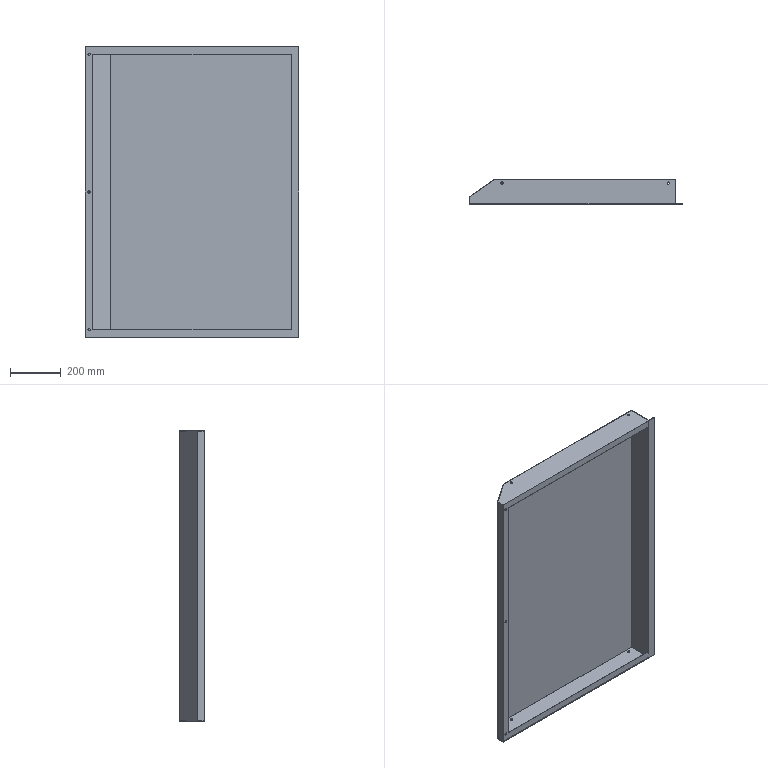Part | SolidWorks | features ICE 5, Extrusion 1, Shell 1 | 1 solid | 37 faces | box 841 x 100 x 1142 mm | volume 2713356 mm3 | plane 19 | cylinder 18 | commonest cylinder face diameters 9 x18
STEP:
#1=CARTESIAN_POINT('',(-2.,84.,482.5));
#2=VERTEX_POINT('',#1);
#3=CARTESIAN_POINT('',(-2.,84.,491.5));
#4=VERTEX_POINT('',#3);
#5=CARTESIAN_POINT('',(-2.,84.,487.));
#6=DIRECTION('',(-1.,0.,0.));
#7=DIRECTION('',(0.,0.,1.));
#8=AXIS2_PLACEMENT_3D('',#5,#6,#7);
#9=CIRCLE('',#8,4.5);
#10=EDGE_CURVE('',#2,#4,#9,.T.);
#11=ORIENTED_EDGE('',*,*,#10,.T.);
#12=CARTESIAN_POINT('',(0.,84.,491.5));
#13=VERTEX_POINT('',#12);
#14=CARTESIAN_POINT('',(-10.,84.,491.5));
#15=DIRECTION('',(1.,0.,0.));
#16=VECTOR('',#15,1000.);
#17=LINE('',#14,#16);
#18=EDGE_CURVE('',#4,#13,#17,.T.);
#19=ORIENTED_EDGE('',*,*,#18,.T.);
#20=CARTESIAN_POINT('',(0.,84.,482.5));
#21=VERTEX_POINT('',#20);
#22=CARTESIAN_POINT('',(0.,84.,487.));
#23=DIRECTION('',(1.,0.,0.));
#24=DIRECTION('',(0.,0.,-1.));
#25=AXIS2_PLACEMENT_3D('',#22,#23,#24);
#26=CIRCLE('',#25,4.5);
#27=EDGE_CURVE('',#13,#21,#26,.T.);
#28=ORIENTED_EDGE('',*,*,#27,.T.);
#29=CARTESIAN_POINT('',(-10.,84.,482.5));
#30=DIRECTION('',(1.,0.,0.));
#31=VECTOR('',#30,1000.);
#32=LINE('',#29,#31);
#33=EDGE_CURVE('',#2,#21,#32,.T.);
#34=ORIENTED_EDGE('',*,*,#33,.F.);
#35=EDGE_LOOP('',(#11,#19,#28,#34));
#36=FACE_OUTER_BOUND('',#35,.T.);
#37=CARTESIAN_POINT('',(-10.,84.,487.));
#38=DIRECTION('',(1.,0.,0.));
#39=DIRECTION('',(0.,0.,-1.));
#40=AXIS2_PLACEMENT_3D('',#37,#38,#39);
#41=CYLINDRICAL_SURFACE('',#40,4.5);
#42=ADVANCED_FACE('',(#36),#41,.F.);
#43=CARTESIAN_POINT('',(-2.,84.,550.5));
#44=VERTEX_POINT('',#43);
#45=CARTESIAN_POINT('',(-2.,84.,559.5));
#46=VERTEX_POINT('',#45);
#47=CARTESIAN_POINT('',(-2.,84.,555.));
#48=DIRECTION('',(-1.,0.,0.));
#49=DIRECTION('',(0.,0.,1.));
#50=AXIS2_PLACEMENT_3D('',#47,#48,#49);
#51=CIRCLE('',#50,4.5);
#52=EDGE_CURVE('',#44,#46,#51,.T.);
#53=ORIENTED_EDGE('',*,*,#52,.T.);
#54=CARTESIAN_POINT('',(0.,84.,559.5));
#55=VERTEX_POINT('',#54);
#56=CARTESIAN_POINT('',(-10.,84.,559.5));
#57=DIRECTION('',(1.,0.,0.));
#58=VECTOR('',#57,1000.);
#59=LINE('',#56,#58);
#60=EDGE_CURVE('',#46,#55,#59,.T.);
#61=ORIENTED_EDGE('',*,*,#60,.T.);
#62=CARTESIAN_POINT('',(0.,84.,550.5));
#63=VERTEX_POINT('',#62);
#64=CARTESIAN_POINT('',(0.,84.,555.));
#65=DIRECTION('',(1.,0.,0.));
#66=DIRECTION('',(0.,0.,-1.));
#67=AXIS2_PLACEMENT_3D('',#64,#65,#66);
#68=CIRCLE('',#67,4.5);
#69=EDGE_CURVE('',#55,#63,#68,.T.);
#70=ORIENTED_EDGE('',*,*,#69,.T.);
#71=CARTESIAN_POINT('',(-10.,84.,550.5));
#72=DIRECTION('',(1.,0.,0.));
#73=VECTOR('',#72,1000.);
#74=LINE('',#71,#73);
#75=EDGE_CURVE('',#44,#63,#74,.T.);
#76=ORIENTED_EDGE('',*,*,#75,.F.);
#77=EDGE_LOOP('',(#53,#61,#70,#76));
#78=FACE_OUTER_BOUND('',#77,.T.);
#79=CARTESIAN_POINT('',(-10.,84.,555.));
#80=DIRECTION('',(1.,0.,0.));
#81=DIRECTION('',(0.,0.,-1.));
#82=AXIS2_PLACEMENT_3D('',#79,#80,#81);
#83=CYLINDRICAL_SURFACE('',#82,4.5);
#84=ADVANCED_FACE('',(#78),#83,.F.);
#85=CARTESIAN_POINT('',(-801.5,2.,0.));
#86=VERTEX_POINT('',#85);
#87=CARTESIAN_POINT('',(-792.5,2.,0.));
#88=VERTEX_POINT('',#87);
#89=CARTESIAN_POINT('',(-797.,2.,0.));
#90=DIRECTION('',(0.,-1.,0.));
#91=DIRECTION('',(1.,0.,0.));
#92=AXIS2_PLACEMENT_3D('',#89,#90,#91);
#93=CIRCLE('',#92,4.5);
#94=EDGE_CURVE('',#86,#88,#93,.T.);
#95=ORIENTED_EDGE('',*,*,#94,.F.);
#96=CARTESIAN_POINT('',(-801.5,0.,0.));
#97=VERTEX_POINT('',#96);
#98=CARTESIAN_POINT('',(-801.5,2.,0.));
#99=DIRECTION('',(0.,-1.,0.));
#100=VECTOR('',#99,1000.);
#101=LINE('',#98,#100);
#102=EDGE_CURVE('',#86,#97,#101,.T.);
#103=ORIENTED_EDGE('',*,*,#102,.T.);
#104=CARTESIAN_POINT('',(-792.5,0.,0.));
#105=VERTEX_POINT('',#104);
#106=CARTESIAN_POINT('',(-797.,0.,0.));
#107=DIRECTION('',(0.,-1.,0.));
#108=DIRECTION('',(1.,0.,0.));
#109=AXIS2_PLACEMENT_3D('',#106,#107,#108);
#110=CIRCLE('',#109,4.5);
#111=EDGE_CURVE('',#97,#105,#110,.T.);
#112=ORIENTED_EDGE('',*,*,#111,.T.);
#113=CARTESIAN_POINT('',(-792.5,2.,0.));
#114=DIRECTION('',(0.,-1.,0.));
#115=VECTOR('',#114,1000.);
#116=LINE('',#113,#115);
#117=EDGE_CURVE('',#88,#105,#116,.T.);
#118=ORIENTED_EDGE('',*,*,#117,.F.);
#119=EDGE_LOOP('',(#95,#103,#112,#118));
#120=FACE_OUTER_BOUND('',#119,.T.);
#121=CARTESIAN_POINT('',(-797.,2.,0.));
#122=DIRECTION('',(0.,-1.,0.));
#123=DIRECTION('',(1.,0.,0.));
#124=AXIS2_PLACEMENT_3D('',#121,#122,#123);
#125=CYLINDRICAL_SURFACE('',#124,4.5);
#126=ADVANCED_FACE('',(#120),#125,.F.);
#127=CARTESIAN_POINT('',(-801.5,2.,-541.));
#128=VERTEX_POINT('',#127);
#129=CARTESIAN_POINT('',(-792.5,2.,-541.));
#130=VERTEX_POINT('',#129);
#131=CARTESIAN_POINT('',(-797.,2.,-541.));
#132=DIRECTION('',(0.,-1.,0.));
#133=DIRECTION('',(1.,0.,0.));
#134=AXIS2_PLACEMENT_3D('',#131,#132,#133);
#135=CIRCLE('',#134,4.5);
#136=EDGE_CURVE('',#128,#130,#135,.T.);
#137=ORIENTED_EDGE('',*,*,#136,.F.);
#138=CARTESIAN_POINT('',(-801.5,0.,-541.));
#139=VERTEX_POINT('',#138);
#140=CARTESIAN_POINT('',(-801.5,2.,-541.));
#141=DIRECTION('',(0.,-1.,0.));
#142=VECTOR('',#141,1000.);
#143=LINE('',#140,#142);
#144=EDGE_CURVE('',#128,#139,#143,.T.);
#145=ORIENTED_EDGE('',*,*,#144,.T.);
#146=CARTESIAN_POINT('',(-792.5,0.,-541.));
#147=VERTEX_POINT('',#146);
#148=CARTESIAN_POINT('',(-797.,0.,-541.));
#149=DIRECTION('',(0.,-1.,0.));
#150=DIRECTION('',(1.,0.,0.));
#151=AXIS2_PLACEMENT_3D('',#148,#149,#150);
#152=CIRCLE('',#151,4.5);
#153=EDGE_CURVE('',#139,#147,#152,.T.);
#154=ORIENTED_EDGE('',*,*,#153,.T.);
#155=CARTESIAN_POINT('',(-792.5,2.,-541.));
#156=DIRECTION('',(0.,-1.,0.));
#157=VECTOR('',#156,1000.);
#158=LINE('',#155,#157);
#159=EDGE_CURVE('',#130,#147,#158,.T.);
#160=ORIENTED_EDGE('',*,*,#159,.F.);
#161=EDGE_LOOP('',(#137,#145,#154,#160));
#162=FACE_OUTER_BOUND('',#161,.T.);
#163=CARTESIAN_POINT('',(-797.,2.,-541.));
#164=DIRECTION('',(0.,-1.,0.));
#165=DIRECTION('',(1.,0.,0.));
#166=AXIS2_PLACEMENT_3D('',#163,#164,#165);
#167=CYLINDRICAL_SURFACE('',#166,4.5);
#168=ADVANCED_FACE('',(#162),#167,.F.);
#169=CARTESIAN_POINT('',(-801.5,2.,541.));
#170=VERTEX_POINT('',#169);
#171=CARTESIAN_POINT('',(-792.5,2.,541.));
#172=VERTEX_POINT('',#171);
#173=CARTESIAN_POINT('',(-797.,2.,541.));
#174=DIRECTION('',(0.,-1.,0.));
#175=DIRECTION('',(1.,0.,0.));
#176=AXIS2_PLACEMENT_3D('',#173,#174,#175);
#177=CIRCLE('',#176,4.5);
#178=EDGE_CURVE('',#170,#172,#177,.T.);
#179=ORIENTED_EDGE('',*,*,#178,.F.);
#180=CARTESIAN_POINT('',(-801.5,0.,541.));
#181=VERTEX_POINT('',#180);
#182=CARTESIAN_POINT('',(-801.5,2.,541.));
#183=DIRECTION('',(0.,-1.,0.));
#184=VECTOR('',#183,1000.);
#185=LINE('',#182,#184);
#186=EDGE_CURVE('',#170,#181,#185,.T.);
#187=ORIENTED_EDGE('',*,*,#186,.T.);
#188=CARTESIAN_POINT('',(-792.5,0.,541.));
#189=VERTEX_POINT('',#188);
#190=CARTESIAN_POINT('',(-797.,0.,541.));
#191=DIRECTION('',(0.,-1.,0.));
#192=DIRECTION('',(1.,0.,0.));
#193=AXIS2_PLACEMENT_3D('',#190,#191,#192);
#194=CIRCLE('',#193,4.5);
#195=EDGE_CURVE('',#181,#189,#194,.T.);
#196=ORIENTED_EDGE('',*,*,#195,.T.);
#197=CARTESIAN_POINT('',(-792.5,2.,541.));
#198=DIRECTION('',(0.,-1.,0.));
#199=VECTOR('',#198,1000.);
#200=LINE('',#197,#199);
#201=EDGE_CURVE('',#172,#189,#200,.T.);
#202=ORIENTED_EDGE('',*,*,#201,.F.);
#203=EDGE_LOOP('',(#179,#187,#196,#202));
#204=FACE_OUTER_BOUND('',#203,.T.);
#205=CARTESIAN_POINT('',(-797.,2.,541.));
#206=DIRECTION('',(0.,-1.,0.));
#207=DIRECTION('',(1.,0.,0.));
#208=AXIS2_PLACEMENT_3D('',#205,#206,#207);
#209=CYLINDRICAL_SURFACE('',#208,4.5);
#210=ADVANCED_FACE('',(#204),#209,.F.);
#211=CARTESIAN_POINT('',(-34.5,84.,569.));
#212=VERTEX_POINT('',#211);
#213=CARTESIAN_POINT('',(-25.5,84.,569.));
#214=VERTEX_POINT('',#213);
#215=CARTESIAN_POINT('',(-30.,84.,569.));
#216=DIRECTION('',(0.,0.,1.));
#217=DIRECTION('',(1.,0.,0.));
#218=AXIS2_PLACEMENT_3D('',#215,#216,#217);
#219=CIRCLE('',#218,4.5);
#220=EDGE_CURVE('',#212,#214,#219,.T.);
#221=ORIENTED_EDGE('',*,*,#220,.F.);
#222=CARTESIAN_POINT('',(-34.5,84.,571.));
#223=VERTEX_POINT('',#222);
#224=CARTESIAN_POINT('',(-34.5,84.,-604.));
#225=DIRECTION('',(0.,0.,1.));
#226=VECTOR('',#225,1000.);
#227=LINE('',#224,#226);
#228=EDGE_CURVE('',#212,#223,#227,.T.);
#229=ORIENTED_EDGE('',*,*,#228,.T.);
#230=CARTESIAN_POINT('',(-25.5,84.,571.));
#231=VERTEX_POINT('',#230);
#232=CARTESIAN_POINT('',(-30.,84.,571.));
#233=DIRECTION('',(0.,0.,1.));
#234=DIRECTION('',(1.,0.,0.));
#235=AXIS2_PLACEMENT_3D('',#232,#233,#234);
#236=CIRCLE('',#235,4.5);
#237=EDGE_CURVE('',#223,#231,#236,.T.);
#238=ORIENTED_EDGE('',*,*,#237,.T.);
#239=CARTESIAN_POINT('',(-25.5,84.,-604.));
#240=DIRECTION('',(0.,0.,1.));
#241=VECTOR('',#240,1000.);
#242=LINE('',#239,#241);
#243=EDGE_CURVE('',#214,#231,#242,.T.);
#244=ORIENTED_EDGE('',*,*,#243,.F.);
#245=EDGE_LOOP('',(#221,#229,#238,#244));
#246=FACE_OUTER_BOUND('',#245,.T.);
#247=CARTESIAN_POINT('',(-30.,84.,-604.));
#248=DIRECTION('',(0.,0.,1.));
#249=DIRECTION('',(1.,0.,0.));
#250=AXIS2_PLACEMENT_3D('',#247,#248,#249);
#251=CYLINDRICAL_SURFACE('',#250,4.5);
#252=ADVANCED_FACE('',(#246),#251,.F.);
#253=CARTESIAN_POINT('',(-34.5,84.,-571.));
#254=VERTEX_POINT('',#253);
#255=CARTESIAN_POINT('',(-25.5,84.,-571.));
#256=VERTEX_POINT('',#255);
#257=CARTESIAN_POINT('',(-30.,84.,-571.));
#258=DIRECTION('',(0.,0.,1.));
#259=DIRECTION('',(1.,0.,0.));
#260=AXIS2_PLACEMENT_3D('',#257,#258,#259);
#261=CIRCLE('',#260,4.5);
#262=EDGE_CURVE('',#254,#256,#261,.T.);
#263=ORIENTED_EDGE('',*,*,#262,.F.);
#264=CARTESIAN_POINT('',(-34.5,84.,-569.));
#265=VERTEX_POINT('',#264);
#266=CARTESIAN_POINT('',(-34.5,84.,-604.));
#267=DIRECTION('',(0.,0.,1.));
#268=VECTOR('',#267,1000.);
#269=LINE('',#266,#268);
#270=EDGE_CURVE('',#254,#265,#269,.T.);
#271=ORIENTED_EDGE('',*,*,#270,.T.);
#272=CARTESIAN_POINT('',(-25.5,84.,-569.));
#273=VERTEX_POINT('',#272);
#274=CARTESIAN_POINT('',(-30.,84.,-569.));
#275=DIRECTION('',(0.,0.,1.));
#276=DIRECTION('',(1.,0.,0.));
#277=AXIS2_PLACEMENT_3D('',#274,#275,#276);
#278=CIRCLE('',#277,4.5);
#279=EDGE_CURVE('',#265,#273,#278,.T.);
#280=ORIENTED_EDGE('',*,*,#279,.T.);
#281=CARTESIAN_POINT('',(-25.5,84.,-604.));
#282=DIRECTION('',(0.,0.,1.));
#283=VECTOR('',#282,1000.);
#284=LINE('',#281,#283);
#285=EDGE_CURVE('',#256,#273,#284,.T.);
#286=ORIENTED_EDGE('',*,*,#285,.F.);
#287=EDGE_LOOP('',(#263,#271,#280,#286));
#288=FACE_OUTER_BOUND('',#287,.T.);
#289=CARTESIAN_POINT('',(-30.,84.,-604.));
#290=DIRECTION('',(0.,0.,1.));
#291=DIRECTION('',(1.,0.,0.));
#292=AXIS2_PLACEMENT_3D('',#289,#290,#291);
#293=CYLINDRICAL_SURFACE('',#292,4.5);
#294=ADVANCED_FACE('',(#288),#293,.F.);
#295=CARTESIAN_POINT('',(-687.53,84.,569.));
#296=VERTEX_POINT('',#295);
#297=CARTESIAN_POINT('',(-678.53,84.,569.));
#298=VERTEX_POINT('',#297);
#299=CARTESIAN_POINT('',(-683.03,84.,569.));
#300=DIRECTION('',(0.,0.,1.));
#301=DIRECTION('',(1.,0.,0.));
#302=AXIS2_PLACEMENT_3D('',#299,#300,#301);
#303=CIRCLE('',#302,4.5);
#304=EDGE_CURVE('',#296,#298,#303,.T.);
#305=ORIENTED_EDGE('',*,*,#304,.F.);
#306=CARTESIAN_POINT('',(-687.53,84.,571.));
#307=VERTEX_POINT('',#306);
#308=CARTESIAN_POINT('',(-687.53,84.,-604.));
#309=DIRECTION('',(0.,0.,1.));
#310=VECTOR('',#309,1000.);
#311=LINE('',#308,#310);
#312=EDGE_CURVE('',#296,#307,#311,.T.);
#313=ORIENTED_EDGE('',*,*,#312,.T.);
#314=CARTESIAN_POINT('',(-678.53,84.,571.));
#315=VERTEX_POINT('',#314);
#316=CARTESIAN_POINT('',(-683.03,84.,571.));
#317=DIRECTION('',(0.,0.,1.));
#318=DIRECTION('',(1.,0.,0.));
#319=AXIS2_PLACEMENT_3D('',#316,#317,#318);
#320=CIRCLE('',#319,4.5);
#321=EDGE_CURVE('',#307,#315,#320,.T.);
#322=ORIENTED_EDGE('',*,*,#321,.T.);
#323=CARTESIAN_POINT('',(-678.53,84.,-604.));
#324=DIRECTION('',(0.,0.,1.));
#325=VECTOR('',#324,1000.);
#326=LINE('',#323,#325);
#327=EDGE_CURVE('',#298,#315,#326,.T.);
#328=ORIENTED_EDGE('',*,*,#327,.F.);
#329=EDGE_LOOP('',(#305,#313,#322,#328));
#330=FACE_OUTER_BOUND('',#329,.T.);
#331=CARTESIAN_POINT('',(-683.03,84.,-604.));
#332=DIRECTION('',(0.,0.,1.));
#333=DIRECTION('',(1.,0.,0.));
#334=AXIS2_PLACEMENT_3D('',#331,#332,#333);
#335=CYLINDRICAL_SURFACE('',#334,4.5);
#336=ADVANCED_FACE('',(#330),#335,.F.);
#337=CARTESIAN_POINT('',(-687.53,84.,-571.));
#338=VERTEX_POINT('',#337);
#339=CARTESIAN_POINT('',(-678.53,84.,-571.));
#340=VERTEX_POINT('',#339);
#341=CARTESIAN_POINT('',(-683.03,84.,-571.));
#342=DIRECTION('',(0.,0.,1.));
#343=DIRECTION('',(1.,0.,0.));
#344=AXIS2_PLACEMENT_3D('',#341,#342,#343);
#345=CIRCLE('',#344,4.5);
#346=EDGE_CURVE('',#338,#340,#345,.T.);
#347=ORIENTED_EDGE('',*,*,#346,.F.);
#348=CARTESIAN_POINT('',(-687.53,84.,-569.));
#349=VERTEX_POINT('',#348);
#350=CARTESIAN_POINT('',(-687.53,84.,-604.));
#351=DIRECTION('',(0.,0.,1.));
#352=VECTOR('',#351,1000.);
#353=LINE('',#350,#352);
#354=EDGE_CURVE('',#338,#349,#353,.T.);
#355=ORIENTED_EDGE('',*,*,#354,.T.);
#356=CARTESIAN_POINT('',(-678.53,84.,-569.));
#357=VERTEX_POINT('',#356);
#358=CARTESIAN_POINT('',(-683.03,84.,-569.));
#359=DIRECTION('',(0.,0.,1.));
#360=DIRECTION('',(1.,0.,0.));
#361=AXIS2_PLACEMENT_3D('',#358,#359,#360);
#362=CIRCLE('',#361,4.5);
#363=EDGE_CURVE('',#349,#357,#362,.T.);
#364=ORIENTED_EDGE('',*,*,#363,.T.);
#365=CARTESIAN_POINT('',(-678.53,84.,-604.));
#366=DIRECTION('',(0.,0.,1.));
#367=VECTOR('',#366,1000.);
#368=LINE('',#365,#367);
#369=EDGE_CURVE('',#340,#357,#368,.T.);
#370=ORIENTED_EDGE('',*,*,#369,.F.);
#371=EDGE_LOOP('',(#347,#355,#364,#370));
#372=FACE_OUTER_BOUND('',#371,.T.);
#373=CARTESIAN_POINT('',(-683.03,84.,-604.));
#374=DIRECTION('',(0.,0.,1.));
#375=DIRECTION('',(1.,0.,0.));
#376=AXIS2_PLACEMENT_3D('',#373,#374,#375);
#377=CYLINDRICAL_SURFACE('',#376,4.5);
#378=ADVANCED_FACE('',(#372),#377,.F.);
#379=CARTESIAN_POINT('',(-811.,28.959,569.));
#380=VERTEX_POINT('',#379);
#381=CARTESIAN_POINT('',(-811.,2.,569.));
#382=VERTEX_POINT('',#381);
#383=CARTESIAN_POINT('',(-811.,0.,569.));
#384=DIRECTION('',(0.,-1.,0.));
#385=VECTOR('',#384,1000.);
#386=LINE('',#383,#385);
#387=EDGE_CURVE('',#380,#382,#386,.T.);
#388=ORIENTED_EDGE('',*,*,#387,.T.);
#389=CARTESIAN_POINT('',(-811.,2.,-569.));
#390=VERTEX_POINT('',#389);
#391=CARTESIAN_POINT('',(-811.,2.,571.));
#392=DIRECTION('',(0.,0.,-1.));
#393=VECTOR('',#392,1000.);
#394=LINE('',#391,#393);
#395=EDGE_CURVE('',#382,#390,#394,.T.);
#396=ORIENTED_EDGE('',*,*,#395,.T.);
#397=CARTESIAN_POINT('',(-811.,28.959,-569.));
#398=VERTEX_POINT('',#397);
#399=CARTESIAN_POINT('',(-811.,0.,-569.));
#400=DIRECTION('',(0.,-1.,0.));
#401=VECTOR('',#400,1000.);
#402=LINE('',#399,#401);
#403=EDGE_CURVE('',#398,#390,#402,.T.);
#404=ORIENTED_EDGE('',*,*,#403,.F.);
#405=CARTESIAN_POINT('',(-811.,28.959,571.));
#406=DIRECTION('',(0.,0.,-1.));
#407=VECTOR('',#406,1000.);
#408=LINE('',#405,#407);
#409=EDGE_CURVE('',#380,#398,#408,.T.);
#410=ORIENTED_EDGE('',*,*,#409,.F.);
#411=EDGE_LOOP('',(#388,#396,#404,#410));
#412=FACE_OUTER_BOUND('',#411,.T.);
#413=CARTESIAN_POINT('',(-811.,0.,571.));
#414=DIRECTION('',(1.,0.,0.));
#415=DIRECTION('',(0.,1.,0.));
#416=AXIS2_PLACEMENT_3D('',#413,#414,#415);
#417=PLANE('',#416);
#418=ADVANCED_FACE('',(#412),#417,.T.);
#419=CARTESIAN_POINT('',(-683.03,84.,569.));
#420=DIRECTION('',(0.,0.,1.));
#421=DIRECTION('',(1.,0.,0.));
#422=AXIS2_PLACEMENT_3D('',#419,#420,#421);
#423=CIRCLE('',#422,4.5);
#424=EDGE_CURVE('',#298,#296,#423,.T.);
#425=ORIENTED_EDGE('',*,*,#424,.T.);
#426=ORIENTED_EDGE('',*,*,#304,.T.);
#427=EDGE_LOOP('',(#425,#426));
#428=FACE_BOUND('',#427,.T.);
#429=CARTESIAN_POINT('',(-30.,84.,569.));
#430=DIRECTION('',(0.,0.,1.));
#431=DIRECTION('',(1.,0.,0.));
#432=AXIS2_PLACEMENT_3D('',#429,#430,#431);
#433=CIRCLE('',#432,4.5);
#434=EDGE_CURVE('',#214,#212,#433,.T.);
#435=ORIENTED_EDGE('',*,*,#434,.T.);
#436=ORIENTED_EDGE('',*,*,#220,.T.);
#437=EDGE_LOOP('',(#435,#436));
#438=FACE_BOUND('',#437,.T.);
#439=CARTESIAN_POINT('',(-2.,2.,569.));
#440=VERTEX_POINT('',#439);
#441=CARTESIAN_POINT('',(0.,2.,569.));
#442=DIRECTION('',(1.,0.,0.));
#443=VECTOR('',#442,1000.);
#444=LINE('',#441,#443);
#445=EDGE_CURVE('',#382,#440,#444,.T.);
#446=ORIENTED_EDGE('',*,*,#445,.F.);
#447=ORIENTED_EDGE('',*,*,#387,.F.);
#448=CARTESIAN_POINT('',(-712.399,98.,569.));
#449=VERTEX_POINT('',#448);
#450=CARTESIAN_POINT('',(-711.882,98.362,569.));
#451=DIRECTION('',(-0.8192,-0.5736,0.));
#452=VECTOR('',#451,1000.);
#453=LINE('',#450,#452);
#454=EDGE_CURVE('',#449,#380,#453,.T.);
#455=ORIENTED_EDGE('',*,*,#454,.F.);
#456=CARTESIAN_POINT('',(-2.,98.,569.));
#457=VERTEX_POINT('',#456);
#458=CARTESIAN_POINT('',(0.,98.,569.));
#459=DIRECTION('',(-1.,0.,0.));
#460=VECTOR('',#459,1000.);
#461=LINE('',#458,#460);
#462=EDGE_CURVE('',#457,#449,#461,.T.);
#463=ORIENTED_EDGE('',*,*,#462,.F.);
#464=CARTESIAN_POINT('',(-2.,0.,569.));
#465=DIRECTION('',(0.,1.,0.));
#466=VECTOR('',#465,1000.);
#467=LINE('',#464,#466);
#468=EDGE_CURVE('',#440,#457,#467,.T.);
#469=ORIENTED_EDGE('',*,*,#468,.F.);
#470=EDGE_LOOP('',(#446,#447,#455,#463,#469));
#471=FACE_OUTER_BOUND('',#470,.T.);
#472=CARTESIAN_POINT('',(0.,100.,569.));
#473=DIRECTION('',(0.,0.,1.));
#474=DIRECTION('',(1.,0.,0.));
#475=AXIS2_PLACEMENT_3D('',#472,#473,#474);
#476=PLANE('',#475);
#477=ADVANCED_FACE('',(#428,#438,#471),#476,.F.);
#478=CARTESIAN_POINT('',(-683.03,84.,-569.));
#479=DIRECTION('',(0.,0.,1.));
#480=DIRECTION('',(1.,0.,0.));
#481=AXIS2_PLACEMENT_3D('',#478,#479,#480);
#482=CIRCLE('',#481,4.5);
#483=EDGE_CURVE('',#357,#349,#482,.T.);
#484=ORIENTED_EDGE('',*,*,#483,.F.);
#485=ORIENTED_EDGE('',*,*,#363,.F.);
#486=EDGE_LOOP('',(#484,#485));
#487=FACE_BOUND('',#486,.T.);
#488=CARTESIAN_POINT('',(-30.,84.,-569.));
#489=DIRECTION('',(0.,0.,1.));
#490=DIRECTION('',(1.,0.,0.));
#491=AXIS2_PLACEMENT_3D('',#488,#489,#490);
#492=CIRCLE('',#491,4.5);
#493=EDGE_CURVE('',#273,#265,#492,.T.);
#494=ORIENTED_EDGE('',*,*,#493,.F.);
#495=ORIENTED_EDGE('',*,*,#279,.F.);
#496=EDGE_LOOP('',(#494,#495));
#497=FACE_BOUND('',#496,.T.);
#498=ORIENTED_EDGE('',*,*,#403,.T.);
#499=CARTESIAN_POINT('',(-2.,2.,-569.));
#500=VERTEX_POINT('',#499);
#501=CARTESIAN_POINT('',(0.,2.,-569.));
#502=DIRECTION('',(1.,0.,0.));
#503=VECTOR('',#502,1000.);
#504=LINE('',#501,#503);
#505=EDGE_CURVE('',#390,#500,#504,.T.);
#506=ORIENTED_EDGE('',*,*,#505,.T.);
#507=CARTESIAN_POINT('',(-2.,98.,-569.));
#508=VERTEX_POINT('',#507);
#509=CARTESIAN_POINT('',(-2.,0.,-569.));
#510=DIRECTION('',(0.,1.,0.));
#511=VECTOR('',#510,1000.);
#512=LINE('',#509,#511);
#513=EDGE_CURVE('',#500,#508,#512,.T.);
#514=ORIENTED_EDGE('',*,*,#513,.T.);
#515=CARTESIAN_POINT('',(-712.399,98.,-569.));
#516=VERTEX_POINT('',#515);
#517=CARTESIAN_POINT('',(0.,98.,-569.));
#518=DIRECTION('',(-1.,0.,0.));
#519=VECTOR('',#518,1000.);
#520=LINE('',#517,#519);
#521=EDGE_CURVE('',#508,#516,#520,.T.);
#522=ORIENTED_EDGE('',*,*,#521,.T.);
#523=CARTESIAN_POINT('',(-711.882,98.362,-569.));
#524=DIRECTION('',(-0.8192,-0.5736,0.));
#525=VECTOR('',#524,1000.);
#526=LINE('',#523,#525);
#527=EDGE_CURVE('',#516,#398,#526,.T.);
#528=ORIENTED_EDGE('',*,*,#527,.T.);
#529=EDGE_LOOP('',(#498,#506,#514,#522,#528));
#530=FACE_OUTER_BOUND('',#529,.T.);
#531=CARTESIAN_POINT('',(0.,100.,-569.));
#532=DIRECTION('',(0.,0.,1.));
#533=DIRECTION('',(1.,0.,0.));
#534=AXIS2_PLACEMENT_3D('',#531,#532,#533);
#535=PLANE('',#534);
#536=ADVANCED_FACE('',(#487,#497,#530),#535,.T.);
#537=CARTESIAN_POINT('',(0.,84.,487.));
#538=DIRECTION('',(1.,0.,0.));
#539=DIRECTION('',(0.,0.,-1.));
#540=AXIS2_PLACEMENT_3D('',#537,#538,#539);
#541=CIRCLE('',#540,4.5);
#542=EDGE_CURVE('',#21,#13,#541,.T.);
#543=ORIENTED_EDGE('',*,*,#542,.F.);
#544=ORIENTED_EDGE('',*,*,#27,.F.);
#545=EDGE_LOOP('',(#543,#544));
#546=FACE_BOUND('',#545,.T.);
#547=CARTESIAN_POINT('',(0.,84.,555.));
#548=DIRECTION('',(1.,0.,0.));
#549=DIRECTION('',(0.,0.,-1.));
#550=AXIS2_PLACEMENT_3D('',#547,#548,#549);
#551=CIRCLE('',#550,4.5);
#552=EDGE_CURVE('',#63,#55,#551,.T.);
#553=ORIENTED_EDGE('',*,*,#552,.F.);
#554=ORIENTED_EDGE('',*,*,#69,.F.);
#555=EDGE_LOOP('',(#553,#554));
#556=FACE_BOUND('',#555,.T.);
#557=CARTESIAN_POINT('',(0.,2.,-571.));
#558=VERTEX_POINT('',#557);
#559=CARTESIAN_POINT('',(0.,2.,571.));
#560=VERTEX_POINT('',#559);
#561=CARTESIAN_POINT('',(0.,2.,571.));
#562=DIRECTION('',(0.,0.,1.));
#563=VECTOR('',#562,1000.);
#564=LINE('',#561,#563);
#565=EDGE_CURVE('',#558,#560,#564,.T.);
#566=ORIENTED_EDGE('',*,*,#565,.F.);
#567=CARTESIAN_POINT('',(0.,100.,-571.));
#568=VERTEX_POINT('',#567);
#569=CARTESIAN_POINT('',(0.,0.,-571.));
#570=DIRECTION('',(0.,1.,0.));
#571=VECTOR('',#570,1000.);
#572=LINE('',#569,#571);
#573=EDGE_CURVE('',#558,#568,#572,.T.);
#574=ORIENTED_EDGE('',*,*,#573,.T.);
#575=CARTESIAN_POINT('',(0.,100.,571.));
#576=VERTEX_POINT('',#575);
#577=CARTESIAN_POINT('',(0.,100.,571.));
#578=DIRECTION('',(0.,0.,-1.));
#579=VECTOR('',#578,1000.);
#580=LINE('',#577,#579);
#581=EDGE_CURVE('',#576,#568,#580,.T.);
#582=ORIENTED_EDGE('',*,*,#581,.F.);
#583=CARTESIAN_POINT('',(0.,0.,571.));
#584=DIRECTION('',(0.,1.,0.));
#585=VECTOR('',#584,1000.);
#586=LINE('',#583,#585);
#587=EDGE_CURVE('',#560,#576,#586,.T.);
#588=ORIENTED_EDGE('',*,*,#587,.F.);
#589=EDGE_LOOP('',(#566,#574,#582,#588));
#590=FACE_OUTER_BOUND('',#589,.T.);
#591=CARTESIAN_POINT('',(0.,0.,571.));
#592=DIRECTION('',(-1.,0.,0.));
#593=DIRECTION('',(0.,0.,1.));
#594=AXIS2_PLACEMENT_3D('',#591,#592,#593);
#595=PLANE('',#594);
#596=ADVANCED_FACE('',(#546,#556,#590),#595,.F.);
#597=CARTESIAN_POINT('',(-797.,0.,0.));
#598=DIRECTION('',(0.,-1.,0.));
#599=DIRECTION('',(1.,0.,0.));
#600=AXIS2_PLACEMENT_3D('',#597,#598,#599);
#601=CIRCLE('',#600,4.5);
#602=EDGE_CURVE('',#105,#97,#601,.T.);
#603=ORIENTED_EDGE('',*,*,#602,.F.);
#604=ORIENTED_EDGE('',*,*,#111,.F.);
#605=EDGE_LOOP('',(#603,#604));
#606=FACE_BOUND('',#605,.T.);
#607=CARTESIAN_POINT('',(-797.,0.,-541.));
#608=DIRECTION('',(0.,-1.,0.));
#609=DIRECTION('',(1.,0.,0.));
#610=AXIS2_PLACEMENT_3D('',#607,#608,#609);
#611=CIRCLE('',#610,4.5);
#612=EDGE_CURVE('',#147,#139,#611,.T.);
#613=ORIENTED_EDGE('',*,*,#612,.F.);
#614=ORIENTED_EDGE('',*,*,#153,.F.);
#615=EDGE_LOOP('',(#613,#614));
#616=FACE_BOUND('',#615,.T.);
#617=CARTESIAN_POINT('',(-797.,0.,541.));
#618=DIRECTION('',(0.,-1.,0.));
#619=DIRECTION('',(1.,0.,0.));
#620=AXIS2_PLACEMENT_3D('',#617,#618,#619);
#621=CIRCLE('',#620,4.5);
#622=EDGE_CURVE('',#189,#181,#621,.T.);
#623=ORIENTED_EDGE('',*,*,#622,.F.);
#624=ORIENTED_EDGE('',*,*,#195,.F.);
#625=EDGE_LOOP('',(#623,#624));
#626=FACE_BOUND('',#625,.T.);
#627=CARTESIAN_POINT('',(-783.,0.,541.));
#628=VERTEX_POINT('',#627);
#629=CARTESIAN_POINT('',(-2.,0.,541.));
#630=VERTEX_POINT('',#629);
#631=CARTESIAN_POINT('',(-783.,0.,541.));
#632=DIRECTION('',(1.,0.,0.));
#633=VECTOR('',#632,1000.);
#634=LINE('',#631,#633);
#635=EDGE_CURVE('',#628,#630,#634,.T.);
#636=ORIENTED_EDGE('',*,*,#635,.T.);
#637=CARTESIAN_POINT('',(-2.,0.,-541.));
#638=VERTEX_POINT('',#637);
#639=CARTESIAN_POINT('',(-2.,0.,571.));
#640=DIRECTION('',(0.,0.,-1.));
#641=VECTOR('',#640,1000.);
#642=LINE('',#639,#641);
#643=EDGE_CURVE('',#630,#638,#642,.T.);
#644=ORIENTED_EDGE('',*,*,#643,.T.);
#645=CARTESIAN_POINT('',(-783.,0.,-541.));
#646=VERTEX_POINT('',#645);
#647=CARTESIAN_POINT('',(-783.,0.,-541.));
#648=DIRECTION('',(-1.,0.,0.));
#649=VECTOR('',#648,1000.);
#650=LINE('',#647,#649);
#651=EDGE_CURVE('',#638,#646,#650,.T.);
#652=ORIENTED_EDGE('',*,*,#651,.T.);
#653=CARTESIAN_POINT('',(-783.,0.,541.));
#654=DIRECTION('',(0.,0.,1.));
#655=VECTOR('',#654,1000.);
#656=LINE('',#653,#655);
#657=EDGE_CURVE('',#646,#628,#656,.T.);
#658=ORIENTED_EDGE('',*,*,#657,.T.);
#659=EDGE_LOOP('',(#636,#644,#652,#658));
#660=FACE_BOUND('',#659,.T.);
#661=CARTESIAN_POINT('',(28.,0.,-571.));
#662=VERTEX_POINT('',#661);
#663=CARTESIAN_POINT('',(28.,0.,571.));
#664=VERTEX_POINT('',#663);
#665=CARTESIAN_POINT('',(28.,0.,571.));
#666=DIRECTION('',(0.,0.,1.));
#667=VECTOR('',#666,1000.);
#668=LINE('',#665,#667);
#669=EDGE_CURVE('',#662,#664,#668,.T.);
#670=ORIENTED_EDGE('',*,*,#669,.T.);
#671=CARTESIAN_POINT('',(-813.,0.,571.));
#672=VERTEX_POINT('',#671);
#673=CARTESIAN_POINT('',(0.,0.,571.));
#674=DIRECTION('',(1.,0.,0.));
#675=VECTOR('',#674,1000.);
#676=LINE('',#673,#675);
#677=EDGE_CURVE('',#672,#664,#676,.T.);
#678=ORIENTED_EDGE('',*,*,#677,.F.);
#679=CARTESIAN_POINT('',(-813.,0.,-571.));
#680=VERTEX_POINT('',#679);
#681=CARTESIAN_POINT('',(-813.,0.,571.));
#682=DIRECTION('',(0.,0.,-1.));
#683=VECTOR('',#682,1000.);
#684=LINE('',#681,#683);
#685=EDGE_CURVE('',#672,#680,#684,.T.);
#686=ORIENTED_EDGE('',*,*,#685,.T.);
#687=CARTESIAN_POINT('',(0.,0.,-571.));
#688=DIRECTION('',(1.,0.,0.));
#689=VECTOR('',#688,1000.);
#690=LINE('',#687,#689);
#691=EDGE_CURVE('',#680,#662,#690,.T.);
#692=ORIENTED_EDGE('',*,*,#691,.T.);
#693=EDGE_LOOP('',(#670,#678,#686,#692));
#694=FACE_OUTER_BOUND('',#693,.T.);
#695=CARTESIAN_POINT('',(0.,0.,571.));
#696=DIRECTION('',(0.,1.,0.));
#697=DIRECTION('',(-1.,0.,0.));
#698=AXIS2_PLACEMENT_3D('',#695,#696,#697);
#699=PLANE('',#698);
#700=ADVANCED_FACE('',(#606,#616,#626,#660,#694),#699,.F.);
#701=CARTESIAN_POINT('',(-713.03,100.,-571.));
#702=VERTEX_POINT('',#701);
#703=CARTESIAN_POINT('',(0.,100.,-571.));
#704=DIRECTION('',(-1.,0.,0.));
#705=VECTOR('',#704,1000.);
#706=LINE('',#703,#705);
#707=EDGE_CURVE('',#568,#702,#706,.T.);
#708=ORIENTED_EDGE('',*,*,#707,.T.);
#709=CARTESIAN_POINT('',(-713.03,100.,571.));
#710=VERTEX_POINT('',#709);
#711=CARTESIAN_POINT('',(-713.03,100.,571.));
#712=DIRECTION('',(0.,0.,-1.));
#713=VECTOR('',#712,1000.);
#714=LINE('',#711,#713);
#715=EDGE_CURVE('',#710,#702,#714,.T.);
#716=ORIENTED_EDGE('',*,*,#715,.F.);
#717=CARTESIAN_POINT('',(0.,100.,571.));
#718=DIRECTION('',(-1.,0.,0.));
#719=VECTOR('',#718,1000.);
#720=LINE('',#717,#719);
#721=EDGE_CURVE('',#576,#710,#720,.T.);
#722=ORIENTED_EDGE('',*,*,#721,.F.);
#723=ORIENTED_EDGE('',*,*,#581,.T.);
#724=EDGE_LOOP('',(#708,#716,#722,#723));
#725=FACE_OUTER_BOUND('',#724,.T.);
#726=CARTESIAN_POINT('',(0.,100.,571.));
#727=DIRECTION('',(0.,-1.,0.));
#728=DIRECTION('',(1.,0.,0.));
#729=AXIS2_PLACEMENT_3D('',#726,#727,#728);
#730=PLANE('',#729);
#731=ADVANCED_FACE('',(#725),#730,.F.);
#732=CARTESIAN_POINT('',(-813.,30.,-571.));
#733=VERTEX_POINT('',#732);
#734=CARTESIAN_POINT('',(-713.03,100.,-571.));
#735=DIRECTION('',(-0.8192,-0.5736,0.));
#736=VECTOR('',#735,1000.);
#737=LINE('',#734,#736);
#738=EDGE_CURVE('',#702,#733,#737,.T.);
#739=ORIENTED_EDGE('',*,*,#738,.T.);
#740=CARTESIAN_POINT('',(-813.,30.,571.));
#741=VERTEX_POINT('',#740);
#742=CARTESIAN_POINT('',(-813.,30.,571.));
#743=DIRECTION('',(0.,0.,-1.));
#744=VECTOR('',#743,1000.);
#745=LINE('',#742,#744);
#746=EDGE_CURVE('',#741,#733,#745,.T.);
#747=ORIENTED_EDGE('',*,*,#746,.F.);
#748=CARTESIAN_POINT('',(-713.03,100.,571.));
#749=DIRECTION('',(-0.8192,-0.5736,0.));
#750=VECTOR('',#749,1000.);
#751=LINE('',#748,#750);
#752=EDGE_CURVE('',#710,#741,#751,.T.);
#753=ORIENTED_EDGE('',*,*,#752,.F.);
#754=ORIENTED_EDGE('',*,*,#715,.T.);
#755=EDGE_LOOP('',(#739,#747,#753,#754));
#756=FACE_OUTER_BOUND('',#755,.T.);
#757=CARTESIAN_POINT('',(-713.03,100.,571.));
#758=DIRECTION('',(0.5736,-0.8192,0.));
#759=DIRECTION('',(0.8192,0.5736,0.));
#760=AXIS2_PLACEMENT_3D('',#757,#758,#759);
#761=PLANE('',#760);
#762=ADVANCED_FACE('',(#756),#761,.F.);
#763=ORIENTED_EDGE('',*,*,#685,.F.);
#764=CARTESIAN_POINT('',(-813.,0.,571.));
#765=DIRECTION('',(0.,-1.,0.));
#766=VECTOR('',#765,1000.);
#767=LINE('',#764,#766);
#768=EDGE_CURVE('',#741,#672,#767,.T.);
#769=ORIENTED_EDGE('',*,*,#768,.F.);
#770=ORIENTED_EDGE('',*,*,#746,.T.);
#771=CARTESIAN_POINT('',(-813.,0.,-571.));
#772=DIRECTION('',(0.,-1.,0.));
#773=VECTOR('',#772,1000.);
#774=LINE('',#771,#773);
#775=EDGE_CURVE('',#733,#680,#774,.T.);
#776=ORIENTED_EDGE('',*,*,#775,.T.);
#777=EDGE_LOOP('',(#763,#769,#770,#776));
#778=FACE_OUTER_BOUND('',#777,.T.);
#779=CARTESIAN_POINT('',(-813.,0.,571.));
#780=DIRECTION('',(1.,0.,0.));
#781=DIRECTION('',(0.,1.,0.));
#782=AXIS2_PLACEMENT_3D('',#779,#780,#781);
#783=PLANE('',#782);
#784=ADVANCED_FACE('',(#778),#783,.F.);
#785=CARTESIAN_POINT('',(28.,2.,571.));
#786=VERTEX_POINT('',#785);
#787=CARTESIAN_POINT('',(-2.,2.,571.));
#788=DIRECTION('',(-1.,0.,0.));
#789=VECTOR('',#788,1000.);
#790=LINE('',#787,#789);
#791=EDGE_CURVE('',#786,#560,#790,.T.);
#792=ORIENTED_EDGE('',*,*,#791,.T.);
#793=ORIENTED_EDGE('',*,*,#587,.T.);
#794=ORIENTED_EDGE('',*,*,#721,.T.);
#795=ORIENTED_EDGE('',*,*,#752,.T.);
#796=ORIENTED_EDGE('',*,*,#768,.T.);
#797=ORIENTED_EDGE('',*,*,#677,.T.);
#798=CARTESIAN_POINT('',(28.,2.,571.));
#799=DIRECTION('',(0.,-1.,0.));
#800=VECTOR('',#799,1000.);
#801=LINE('',#798,#800);
#802=EDGE_CURVE('',#786,#664,#801,.T.);
#803=ORIENTED_EDGE('',*,*,#802,.F.);
#804=EDGE_LOOP('',(#792,#793,#794,#795,#796,#797,#803));
#805=FACE_OUTER_BOUND('',#804,.T.);
#806=CARTESIAN_POINT('',(-683.03,84.,571.));
#807=DIRECTION('',(0.,0.,1.));
#808=DIRECTION('',(1.,0.,0.));
#809=AXIS2_PLACEMENT_3D('',#806,#807,#808);
#810=CIRCLE('',#809,4.5);
#811=EDGE_CURVE('',#315,#307,#810,.T.);
#812=ORIENTED_EDGE('',*,*,#811,.F.);
#813=ORIENTED_EDGE('',*,*,#321,.F.);
#814=EDGE_LOOP('',(#812,#813));
#815=FACE_BOUND('',#814,.T.);
#816=CARTESIAN_POINT('',(-30.,84.,571.));
#817=DIRECTION('',(0.,0.,1.));
#818=DIRECTION('',(1.,0.,0.));
#819=AXIS2_PLACEMENT_3D('',#816,#817,#818);
#820=CIRCLE('',#819,4.5);
#821=EDGE_CURVE('',#231,#223,#820,.T.);
#822=ORIENTED_EDGE('',*,*,#821,.F.);
#823=ORIENTED_EDGE('',*,*,#237,.F.);
#824=EDGE_LOOP('',(#822,#823));
#825=FACE_BOUND('',#824,.T.);
#826=CARTESIAN_POINT('',(0.,100.,571.));
#827=DIRECTION('',(0.,0.,1.));
#828=DIRECTION('',(1.,0.,0.));
#829=AXIS2_PLACEMENT_3D('',#826,#827,#828);
#830=PLANE('',#829);
#831=ADVANCED_FACE('',(#805,#815,#825),#830,.T.);
#832=CARTESIAN_POINT('',(28.,2.,-571.));
#833=VERTEX_POINT('',#832);
#834=CARTESIAN_POINT('',(28.,2.,-571.));
#835=DIRECTION('',(0.,-1.,0.));
#836=VECTOR('',#835,1000.);
#837=LINE('',#834,#836);
#838=EDGE_CURVE('',#833,#662,#837,.T.);
#839=ORIENTED_EDGE('',*,*,#838,.T.);
#840=ORIENTED_EDGE('',*,*,#691,.F.);
#841=ORIENTED_EDGE('',*,*,#775,.F.);
#842=ORIENTED_EDGE('',*,*,#738,.F.);
#843=ORIENTED_EDGE('',*,*,#707,.F.);
#844=ORIENTED_EDGE('',*,*,#573,.F.);
#845=CARTESIAN_POINT('',(-2.,2.,-571.));
#846=DIRECTION('',(1.,0.,0.));
#847=VECTOR('',#846,1000.);
#848=LINE('',#845,#847);
#849=EDGE_CURVE('',#558,#833,#848,.T.);
#850=ORIENTED_EDGE('',*,*,#849,.T.);
#851=EDGE_LOOP('',(#839,#840,#841,#842,#843,#844,#850));
#852=FACE_OUTER_BOUND('',#851,.T.);
#853=CARTESIAN_POINT('',(-683.03,84.,-571.));
#854=DIRECTION('',(0.,0.,1.));
#855=DIRECTION('',(1.,0.,0.));
#856=AXIS2_PLACEMENT_3D('',#853,#854,#855);
#857=CIRCLE('',#856,4.5);
#858=EDGE_CURVE('',#340,#338,#857,.T.);
#859=ORIENTED_EDGE('',*,*,#858,.T.);
#860=ORIENTED_EDGE('',*,*,#346,.T.);
#861=EDGE_LOOP('',(#859,#860));
#862=FACE_BOUND('',#861,.T.);
#863=CARTESIAN_POINT('',(-30.,84.,-571.));
#864=DIRECTION('',(0.,0.,1.));
#865=DIRECTION('',(1.,0.,0.));
#866=AXIS2_PLACEMENT_3D('',#863,#864,#865);
#867=CIRCLE('',#866,4.5);
#868=EDGE_CURVE('',#256,#254,#867,.T.);
#869=ORIENTED_EDGE('',*,*,#868,.T.);
#870=ORIENTED_EDGE('',*,*,#262,.T.);
#871=EDGE_LOOP('',(#869,#870));
#872=FACE_BOUND('',#871,.T.);
#873=CARTESIAN_POINT('',(0.,100.,-571.));
#874=DIRECTION('',(0.,0.,1.));
#875=DIRECTION('',(1.,0.,0.));
#876=AXIS2_PLACEMENT_3D('',#873,#874,#875);
#877=PLANE('',#876);
#878=ADVANCED_FACE('',(#852,#862,#872),#877,.F.);
#879=ORIENTED_EDGE('',*,*,#10,.F.);
#880=CARTESIAN_POINT('',(-2.,84.,487.));
#881=DIRECTION('',(-1.,0.,0.));
#882=DIRECTION('',(0.,0.,1.));
#883=AXIS2_PLACEMENT_3D('',#880,#881,#882);
#884=CIRCLE('',#883,4.5);
#885=EDGE_CURVE('',#4,#2,#884,.T.);
#886=ORIENTED_EDGE('',*,*,#885,.F.);
#887=EDGE_LOOP('',(#879,#886));
#888=FACE_BOUND('',#887,.T.);
#889=ORIENTED_EDGE('',*,*,#52,.F.);
#890=CARTESIAN_POINT('',(-2.,84.,555.));
#891=DIRECTION('',(-1.,0.,0.));
#892=DIRECTION('',(0.,0.,1.));
#893=AXIS2_PLACEMENT_3D('',#890,#891,#892);
#894=CIRCLE('',#893,4.5);
#895=EDGE_CURVE('',#46,#44,#894,.T.);
#896=ORIENTED_EDGE('',*,*,#895,.F.);
#897=EDGE_LOOP('',(#889,#896));
#898=FACE_BOUND('',#897,.T.);
#899=CARTESIAN_POINT('',(-2.,2.,-541.));
#900=VERTEX_POINT('',#899);
#901=CARTESIAN_POINT('',(-2.,0.,-541.));
#902=DIRECTION('',(0.,1.,0.));
#903=VECTOR('',#902,1000.);
#904=LINE('',#901,#903);
#905=EDGE_CURVE('',#638,#900,#904,.T.);
#906=ORIENTED_EDGE('',*,*,#905,.F.);
#907=ORIENTED_EDGE('',*,*,#643,.F.);
#908=CARTESIAN_POINT('',(-2.,2.,541.));
#909=VERTEX_POINT('',#908);
#910=CARTESIAN_POINT('',(-2.,0.,541.));
#911=DIRECTION('',(0.,-1.,0.));
#912=VECTOR('',#911,1000.);
#913=LINE('',#910,#912);
#914=EDGE_CURVE('',#909,#630,#913,.T.);
#915=ORIENTED_EDGE('',*,*,#914,.F.);
#916=CARTESIAN_POINT('',(-2.,2.,571.));
#917=DIRECTION('',(0.,0.,1.));
#918=VECTOR('',#917,1000.);
#919=LINE('',#916,#918);
#920=EDGE_CURVE('',#909,#440,#919,.T.);
#921=ORIENTED_EDGE('',*,*,#920,.T.);
#922=ORIENTED_EDGE('',*,*,#468,.T.);
#923=CARTESIAN_POINT('',(-2.,98.,571.));
#924=DIRECTION('',(0.,0.,-1.));
#925=VECTOR('',#924,1000.);
#926=LINE('',#923,#925);
#927=EDGE_CURVE('',#457,#508,#926,.T.);
#928=ORIENTED_EDGE('',*,*,#927,.T.);
#929=ORIENTED_EDGE('',*,*,#513,.F.);
#930=CARTESIAN_POINT('',(-2.,2.,571.));
#931=DIRECTION('',(0.,0.,1.));
#932=VECTOR('',#931,1000.);
#933=LINE('',#930,#932);
#934=EDGE_CURVE('',#500,#900,#933,.T.);
#935=ORIENTED_EDGE('',*,*,#934,.T.);
#936=EDGE_LOOP('',(#906,#907,#915,#921,#922,#928,#929,#935));
#937=FACE_OUTER_BOUND('',#936,.T.);
#938=CARTESIAN_POINT('',(-2.,0.,571.));
#939=DIRECTION('',(-1.,0.,0.));
#940=DIRECTION('',(0.,0.,1.));
#941=AXIS2_PLACEMENT_3D('',#938,#939,#940);
#942=PLANE('',#941);
#943=ADVANCED_FACE('',(#888,#898,#937),#942,.T.);
#944=ORIENTED_EDGE('',*,*,#521,.F.);
#945=ORIENTED_EDGE('',*,*,#927,.F.);
#946=ORIENTED_EDGE('',*,*,#462,.T.);
#947=CARTESIAN_POINT('',(-712.399,98.,571.));
#948=DIRECTION('',(0.,0.,-1.));
#949=VECTOR('',#948,1000.);
#950=LINE('',#947,#949);
#951=EDGE_CURVE('',#449,#516,#950,.T.);
#952=ORIENTED_EDGE('',*,*,#951,.T.);
#953=EDGE_LOOP('',(#944,#945,#946,#952));
#954=FACE_OUTER_BOUND('',#953,.T.);
#955=CARTESIAN_POINT('',(0.,98.,571.));
#956=DIRECTION('',(0.,-1.,0.));
#957=DIRECTION('',(1.,0.,0.));
#958=AXIS2_PLACEMENT_3D('',#955,#956,#957);
#959=PLANE('',#958);
#960=ADVANCED_FACE('',(#954),#959,.T.);
#961=ORIENTED_EDGE('',*,*,#527,.F.);
#962=ORIENTED_EDGE('',*,*,#951,.F.);
#963=ORIENTED_EDGE('',*,*,#454,.T.);
#964=ORIENTED_EDGE('',*,*,#409,.T.);
#965=EDGE_LOOP('',(#961,#962,#963,#964));
#966=FACE_OUTER_BOUND('',#965,.T.);
#967=CARTESIAN_POINT('',(-711.882,98.362,571.));
#968=DIRECTION('',(0.5736,-0.8192,0.));
#969=DIRECTION('',(0.8192,0.5736,0.));
#970=AXIS2_PLACEMENT_3D('',#967,#968,#969);
#971=PLANE('',#970);
#972=ADVANCED_FACE('',(#966),#971,.T.);
#973=ORIENTED_EDGE('',*,*,#849,.F.);
#974=ORIENTED_EDGE('',*,*,#565,.T.);
#975=ORIENTED_EDGE('',*,*,#791,.F.);
#976=CARTESIAN_POINT('',(28.,2.,571.));
#977=DIRECTION('',(0.,0.,1.));
#978=VECTOR('',#977,1000.);
#979=LINE('',#976,#978);
#980=EDGE_CURVE('',#833,#786,#979,.T.);
#981=ORIENTED_EDGE('',*,*,#980,.F.);
#982=EDGE_LOOP('',(#973,#974,#975,#981));
#983=FACE_OUTER_BOUND('',#982,.T.);
#984=CARTESIAN_POINT('',(-2.,2.,-571.));
#985=DIRECTION('',(0.,-1.,0.));
#986=DIRECTION('',(1.,0.,0.));
#987=AXIS2_PLACEMENT_3D('',#984,#985,#986);
#988=PLANE('',#987);
#989=ADVANCED_FACE('',(#983),#988,.F.);
#990=ORIENTED_EDGE('',*,*,#669,.F.);
#991=ORIENTED_EDGE('',*,*,#838,.F.);
#992=ORIENTED_EDGE('',*,*,#980,.T.);
#993=ORIENTED_EDGE('',*,*,#802,.T.);
#994=EDGE_LOOP('',(#990,#991,#992,#993));
#995=FACE_OUTER_BOUND('',#994,.T.);
#996=CARTESIAN_POINT('',(28.,2.,571.));
#997=DIRECTION('',(1.,0.,0.));
#998=DIRECTION('',(0.,1.,0.));
#999=AXIS2_PLACEMENT_3D('',#996,#997,#998);
#1000=PLANE('',#999);
#1001=ADVANCED_FACE('',(#995),#1000,.T.);
#1002=ORIENTED_EDGE('',*,*,#354,.F.);
#1003=ORIENTED_EDGE('',*,*,#858,.F.);
#1004=ORIENTED_EDGE('',*,*,#369,.T.);
#1005=ORIENTED_EDGE('',*,*,#483,.T.);
#1006=EDGE_LOOP('',(#1002,#1003,#1004,#1005));
#1007=FACE_OUTER_BOUND('',#1006,.T.);
#1008=CARTESIAN_POINT('',(-683.03,84.,-604.));
#1009=DIRECTION('',(0.,0.,1.));
#1010=DIRECTION('',(1.,0.,0.));
#1011=AXIS2_PLACEMENT_3D('',#1008,#1009,#1010);
#1012=CYLINDRICAL_SURFACE('',#1011,4.5);
#1013=ADVANCED_FACE('',(#1007),#1012,.F.);
#1014=ORIENTED_EDGE('',*,*,#312,.F.);
#1015=ORIENTED_EDGE('',*,*,#424,.F.);
#1016=ORIENTED_EDGE('',*,*,#327,.T.);
#1017=ORIENTED_EDGE('',*,*,#811,.T.);
#1018=EDGE_LOOP('',(#1014,#1015,#1016,#1017));
#1019=FACE_OUTER_BOUND('',#1018,.T.);
#1020=CARTESIAN_POINT('',(-683.03,84.,-604.));
#1021=DIRECTION('',(0.,0.,1.));
#1022=DIRECTION('',(1.,0.,0.));
#1023=AXIS2_PLACEMENT_3D('',#1020,#1021,#1022);
#1024=CYLINDRICAL_SURFACE('',#1023,4.5);
#1025=ADVANCED_FACE('',(#1019),#1024,.F.);
#1026=ORIENTED_EDGE('',*,*,#270,.F.);
#1027=ORIENTED_EDGE('',*,*,#868,.F.);
#1028=ORIENTED_EDGE('',*,*,#285,.T.);
#1029=ORIENTED_EDGE('',*,*,#493,.T.);
#1030=EDGE_LOOP('',(#1026,#1027,#1028,#1029));
#1031=FACE_OUTER_BOUND('',#1030,.T.);
#1032=CARTESIAN_POINT('',(-30.,84.,-604.));
#1033=DIRECTION('',(0.,0.,1.));
#1034=DIRECTION('',(1.,0.,0.));
#1035=AXIS2_PLACEMENT_3D('',#1032,#1033,#1034);
#1036=CYLINDRICAL_SURFACE('',#1035,4.5);
#1037=ADVANCED_FACE('',(#1031),#1036,.F.);
#1038=ORIENTED_EDGE('',*,*,#228,.F.);
#1039=ORIENTED_EDGE('',*,*,#434,.F.);
#1040=ORIENTED_EDGE('',*,*,#243,.T.);
#1041=ORIENTED_EDGE('',*,*,#821,.T.);
#1042=EDGE_LOOP('',(#1038,#1039,#1040,#1041));
#1043=FACE_OUTER_BOUND('',#1042,.T.);
#1044=CARTESIAN_POINT('',(-30.,84.,-604.));
#1045=DIRECTION('',(0.,0.,1.));
#1046=DIRECTION('',(1.,0.,0.));
#1047=AXIS2_PLACEMENT_3D('',#1044,#1045,#1046);
#1048=CYLINDRICAL_SURFACE('',#1047,4.5);
#1049=ADVANCED_FACE('',(#1043),#1048,.F.);
#1050=CARTESIAN_POINT('',(-783.,2.,541.));
#1051=VERTEX_POINT('',#1050);
#1052=CARTESIAN_POINT('',(-783.,2.,541.));
#1053=DIRECTION('',(1.,0.,0.));
#1054=VECTOR('',#1053,1000.);
#1055=LINE('',#1052,#1054);
#1056=EDGE_CURVE('',#1051,#909,#1055,.T.);
#1057=ORIENTED_EDGE('',*,*,#1056,.T.);
#1058=ORIENTED_EDGE('',*,*,#914,.T.);
#1059=ORIENTED_EDGE('',*,*,#635,.F.);
#1060=CARTESIAN_POINT('',(-783.,2.,541.));
#1061=DIRECTION('',(0.,-1.,0.));
#1062=VECTOR('',#1061,1000.);
#1063=LINE('',#1060,#1062);
#1064=EDGE_CURVE('',#1051,#628,#1063,.T.);
#1065=ORIENTED_EDGE('',*,*,#1064,.F.);
#1066=EDGE_LOOP('',(#1057,#1058,#1059,#1065));
#1067=FACE_OUTER_BOUND('',#1066,.T.);
#1068=CARTESIAN_POINT('',(-783.,2.,541.));
#1069=DIRECTION('',(0.,0.,-1.));
#1070=DIRECTION('',(-1.,0.,0.));
#1071=AXIS2_PLACEMENT_3D('',#1068,#1069,#1070);
#1072=PLANE('',#1071);
#1073=ADVANCED_FACE('',(#1067),#1072,.T.);
#1074=ORIENTED_EDGE('',*,*,#657,.F.);
#1075=CARTESIAN_POINT('',(-783.,2.,-541.));
#1076=VERTEX_POINT('',#1075);
#1077=CARTESIAN_POINT('',(-783.,2.,-541.));
#1078=DIRECTION('',(0.,-1.,0.));
#1079=VECTOR('',#1078,1000.);
#1080=LINE('',#1077,#1079);
#1081=EDGE_CURVE('',#1076,#646,#1080,.T.);
#1082=ORIENTED_EDGE('',*,*,#1081,.F.);
#1083=CARTESIAN_POINT('',(-783.,2.,541.));
#1084=DIRECTION('',(0.,0.,1.));
#1085=VECTOR('',#1084,1000.);
#1086=LINE('',#1083,#1085);
#1087=EDGE_CURVE('',#1076,#1051,#1086,.T.);
#1088=ORIENTED_EDGE('',*,*,#1087,.T.);
#1089=ORIENTED_EDGE('',*,*,#1064,.T.);
#1090=EDGE_LOOP('',(#1074,#1082,#1088,#1089));
#1091=FACE_OUTER_BOUND('',#1090,.T.);
#1092=CARTESIAN_POINT('',(-783.,2.,541.));
#1093=DIRECTION('',(1.,0.,0.));
#1094=DIRECTION('',(0.,1.,0.));
#1095=AXIS2_PLACEMENT_3D('',#1092,#1093,#1094);
#1096=PLANE('',#1095);
#1097=ADVANCED_FACE('',(#1091),#1096,.T.);
#1098=ORIENTED_EDGE('',*,*,#651,.F.);
#1099=ORIENTED_EDGE('',*,*,#905,.T.);
#1100=CARTESIAN_POINT('',(-783.,2.,-541.));
#1101=DIRECTION('',(-1.,0.,0.));
#1102=VECTOR('',#1101,1000.);
#1103=LINE('',#1100,#1102);
#1104=EDGE_CURVE('',#900,#1076,#1103,.T.);
#1105=ORIENTED_EDGE('',*,*,#1104,.T.);
#1106=ORIENTED_EDGE('',*,*,#1081,.T.);
#1107=EDGE_LOOP('',(#1098,#1099,#1105,#1106));
#1108=FACE_OUTER_BOUND('',#1107,.T.);
#1109=CARTESIAN_POINT('',(-783.,2.,-541.));
#1110=DIRECTION('',(0.,0.,1.));
#1111=DIRECTION('',(1.,0.,0.));
#1112=AXIS2_PLACEMENT_3D('',#1109,#1110,#1111);
#1113=PLANE('',#1112);
#1114=ADVANCED_FACE('',(#1108),#1113,.T.);
#1115=CARTESIAN_POINT('',(-797.,2.,0.));
#1116=DIRECTION('',(0.,-1.,0.));
#1117=DIRECTION('',(1.,0.,0.));
#1118=AXIS2_PLACEMENT_3D('',#1115,#1116,#1117);
#1119=CIRCLE('',#1118,4.5);
#1120=EDGE_CURVE('',#88,#86,#1119,.T.);
#1121=ORIENTED_EDGE('',*,*,#1120,.T.);
#1122=ORIENTED_EDGE('',*,*,#94,.T.);
#1123=EDGE_LOOP('',(#1121,#1122));
#1124=FACE_BOUND('',#1123,.T.);
#1125=CARTESIAN_POINT('',(-797.,2.,-541.));
#1126=DIRECTION('',(0.,-1.,0.));
#1127=DIRECTION('',(1.,0.,0.));
#1128=AXIS2_PLACEMENT_3D('',#1125,#1126,#1127);
#1129=CIRCLE('',#1128,4.5);
#1130=EDGE_CURVE('',#130,#128,#1129,.T.);
#1131=ORIENTED_EDGE('',*,*,#1130,.T.);
#1132=ORIENTED_EDGE('',*,*,#136,.T.);
#1133=EDGE_LOOP('',(#1131,#1132));
#1134=FACE_BOUND('',#1133,.T.);
#1135=CARTESIAN_POINT('',(-797.,2.,541.));
#1136=DIRECTION('',(0.,-1.,0.));
#1137=DIRECTION('',(1.,0.,0.));
#1138=AXIS2_PLACEMENT_3D('',#1135,#1136,#1137);
#1139=CIRCLE('',#1138,4.5);
#1140=EDGE_CURVE('',#172,#170,#1139,.T.);
#1141=ORIENTED_EDGE('',*,*,#1140,.T.);
#1142=ORIENTED_EDGE('',*,*,#178,.T.);
#1143=EDGE_LOOP('',(#1141,#1142));
#1144=FACE_BOUND('',#1143,.T.);
#1145=ORIENTED_EDGE('',*,*,#920,.F.);
#1146=ORIENTED_EDGE('',*,*,#1056,.F.);
#1147=ORIENTED_EDGE('',*,*,#1087,.F.);
#1148=ORIENTED_EDGE('',*,*,#1104,.F.);
#1149=ORIENTED_EDGE('',*,*,#934,.F.);
#1150=ORIENTED_EDGE('',*,*,#505,.F.);
#1151=ORIENTED_EDGE('',*,*,#395,.F.);
#1152=ORIENTED_EDGE('',*,*,#445,.T.);
#1153=EDGE_LOOP('',(#1145,#1146,#1147,#1148,#1149,#1150,#1151,#1152));
#1154=FACE_OUTER_BOUND('',#1153,.T.);
#1155=CARTESIAN_POINT('',(-813.,2.,-571.));
#1156=DIRECTION('',(0.,-1.,0.));
#1157=DIRECTION('',(1.,0.,0.));
#1158=AXIS2_PLACEMENT_3D('',#1155,#1156,#1157);
#1159=PLANE('',#1158);
#1160=ADVANCED_FACE('',(#1124,#1134,#1144,#1154),#1159,.F.);
#1161=ORIENTED_EDGE('',*,*,#186,.F.);
#1162=ORIENTED_EDGE('',*,*,#1140,.F.);
#1163=ORIENTED_EDGE('',*,*,#201,.T.);
#1164=ORIENTED_EDGE('',*,*,#622,.T.);
#1165=EDGE_LOOP('',(#1161,#1162,#1163,#1164));
#1166=FACE_OUTER_BOUND('',#1165,.T.);
#1167=CARTESIAN_POINT('',(-797.,2.,541.));
#1168=DIRECTION('',(0.,-1.,0.));
#1169=DIRECTION('',(1.,0.,0.));
#1170=AXIS2_PLACEMENT_3D('',#1167,#1168,#1169);
#1171=CYLINDRICAL_SURFACE('',#1170,4.5);
#1172=ADVANCED_FACE('',(#1166),#1171,.F.);
#1173=ORIENTED_EDGE('',*,*,#144,.F.);
#1174=ORIENTED_EDGE('',*,*,#1130,.F.);
#1175=ORIENTED_EDGE('',*,*,#159,.T.);
#1176=ORIENTED_EDGE('',*,*,#612,.T.);
#1177=EDGE_LOOP('',(#1173,#1174,#1175,#1176));
#1178=FACE_OUTER_BOUND('',#1177,.T.);
#1179=CARTESIAN_POINT('',(-797.,2.,-541.));
#1180=DIRECTION('',(0.,-1.,0.));
#1181=DIRECTION('',(1.,0.,0.));
#1182=AXIS2_PLACEMENT_3D('',#1179,#1180,#1181);
#1183=CYLINDRICAL_SURFACE('',#1182,4.5);
#1184=ADVANCED_FACE('',(#1178),#1183,.F.);
#1185=ORIENTED_EDGE('',*,*,#102,.F.);
#1186=ORIENTED_EDGE('',*,*,#1120,.F.);
#1187=ORIENTED_EDGE('',*,*,#117,.T.);
#1188=ORIENTED_EDGE('',*,*,#602,.T.);
#1189=EDGE_LOOP('',(#1185,#1186,#1187,#1188));
#1190=FACE_OUTER_BOUND('',#1189,.T.);
#1191=CARTESIAN_POINT('',(-797.,2.,0.));
#1192=DIRECTION('',(0.,-1.,0.));
#1193=DIRECTION('',(1.,0.,0.));
#1194=AXIS2_PLACEMENT_3D('',#1191,#1192,#1193);
#1195=CYLINDRICAL_SURFACE('',#1194,4.5);
#1196=ADVANCED_FACE('',(#1190),#1195,.F.);
#1197=ORIENTED_EDGE('',*,*,#60,.F.);
#1198=ORIENTED_EDGE('',*,*,#895,.T.);
#1199=ORIENTED_EDGE('',*,*,#75,.T.);
#1200=ORIENTED_EDGE('',*,*,#552,.T.);
#1201=EDGE_LOOP('',(#1197,#1198,#1199,#1200));
#1202=FACE_OUTER_BOUND('',#1201,.T.);
#1203=CARTESIAN_POINT('',(-10.,84.,555.));
#1204=DIRECTION('',(1.,0.,0.));
#1205=DIRECTION('',(0.,0.,-1.));
#1206=AXIS2_PLACEMENT_3D('',#1203,#1204,#1205);
#1207=CYLINDRICAL_SURFACE('',#1206,4.5);
#1208=ADVANCED_FACE('',(#1202),#1207,.F.);
#1209=ORIENTED_EDGE('',*,*,#18,.F.);
#1210=ORIENTED_EDGE('',*,*,#885,.T.);
#1211=ORIENTED_EDGE('',*,*,#33,.T.);
#1212=ORIENTED_EDGE('',*,*,#542,.T.);
#1213=EDGE_LOOP('',(#1209,#1210,#1211,#1212));
#1214=FACE_OUTER_BOUND('',#1213,.T.);
#1215=CARTESIAN_POINT('',(-10.,84.,487.));
#1216=DIRECTION('',(1.,0.,0.));
#1217=DIRECTION('',(0.,0.,-1.));
#1218=AXIS2_PLACEMENT_3D('',#1215,#1216,#1217);
#1219=CYLINDRICAL_SURFACE('',#1218,4.5);
#1220=ADVANCED_FACE('',(#1214),#1219,.F.);
#1221=CLOSED_SHELL('',(#42,#84,#126,#168,#210,#252,#294,#336,#378,#418,#477,#536,#596,#700,#731,#762,#784,#831,#878,#943,#960,#972,#989,#1001,#1013,#1025,#1037,#1049,#1073,#1097,#1114,#1160,#1172,#1184,#1196,#1208,#1220));
#1222=MANIFOLD_SOLID_BREP('',#1221);
#1223=CARTESIAN_POINT('',(0.,0.,0.));
#1224=DIRECTION('',(0.,0.,1.));
#1225=DIRECTION('',(1.,0.,0.));
#1226=AXIS2_PLACEMENT_3D('',#1223,#1224,#1225);
#1227=(LENGTH_UNIT()NAMED_UNIT(*)SI_UNIT(.MILLI.,.METRE.));
#1228=UNCERTAINTY_MEASURE_WITH_UNIT(LENGTH_MEASURE(0.00001),#1227,'','');
#1229=(NAMED_UNIT(*)PLANE_ANGLE_UNIT()SI_UNIT($,.RADIAN.));
#1230=(NAMED_UNIT(*)SI_UNIT($,.STERADIAN.)SOLID_ANGLE_UNIT());
#1231=(GEOMETRIC_REPRESENTATION_CONTEXT(3)GLOBAL_UNCERTAINTY_ASSIGNED_CONTEXT((#1228))GLOBAL_UNIT_ASSIGNED_CONTEXT((#1227,#1229,#1230))REPRESENTATION_CONTEXT('',''));
#1232=ADVANCED_BREP_SHAPE_REPRESENTATION('',(#1222,#1226),#1231);